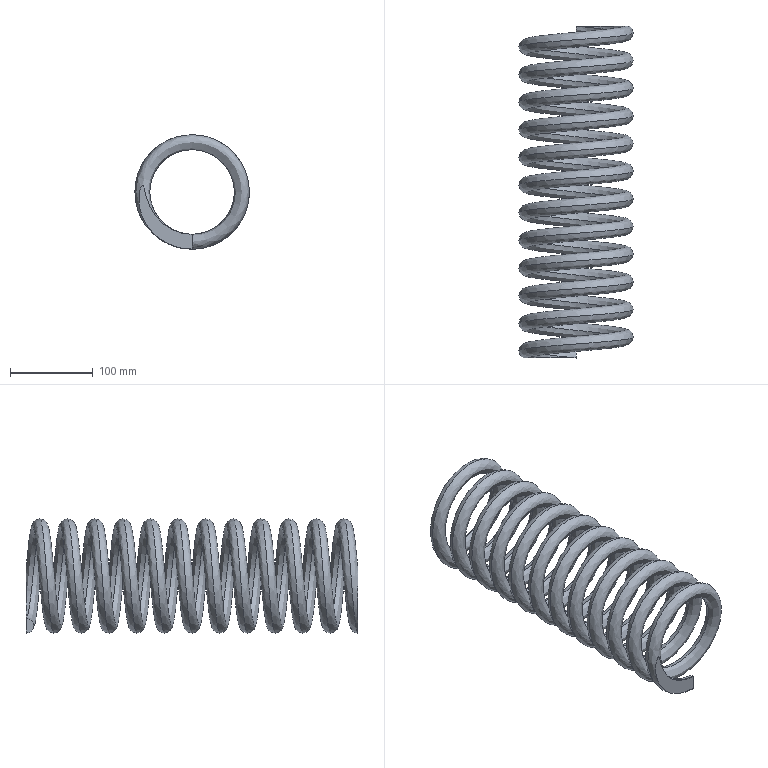Part | SolidWorks | features ICE 1, Sweep 1 | 1 solid | 6 faces | box 138 x 400.231 x 138 mm | volume 1136867 mm3 | plane 4 | spline 2